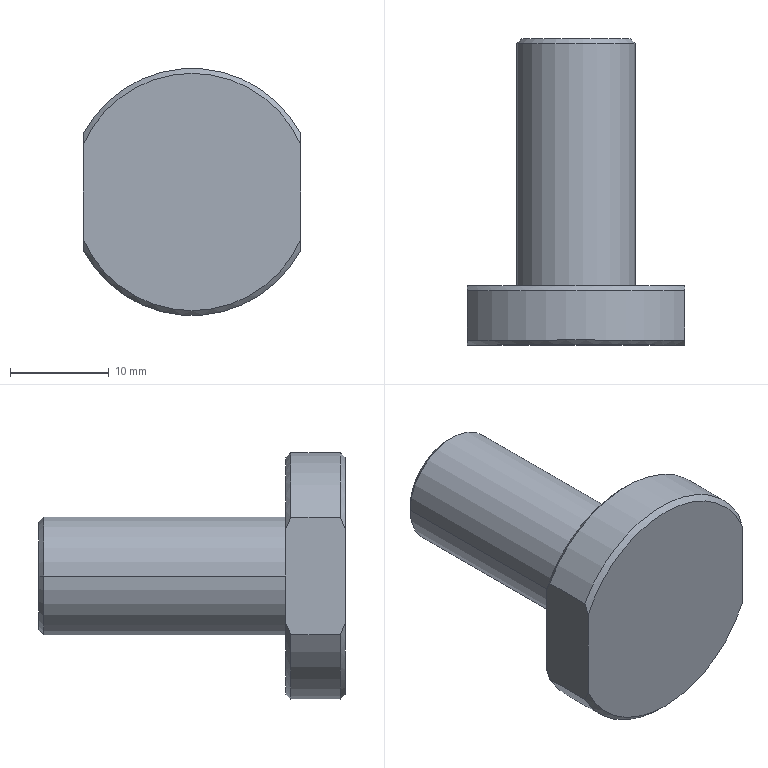Part | STEP file | Polisher upper hinge | 1 solid | 19 faces | box 22 x 31 x 25 mm | volume 5247 mm3 | cone 8 | cylinder 6 | plane 5 | commonest cylinder face diameters 5 x2 12 x2 25 x2